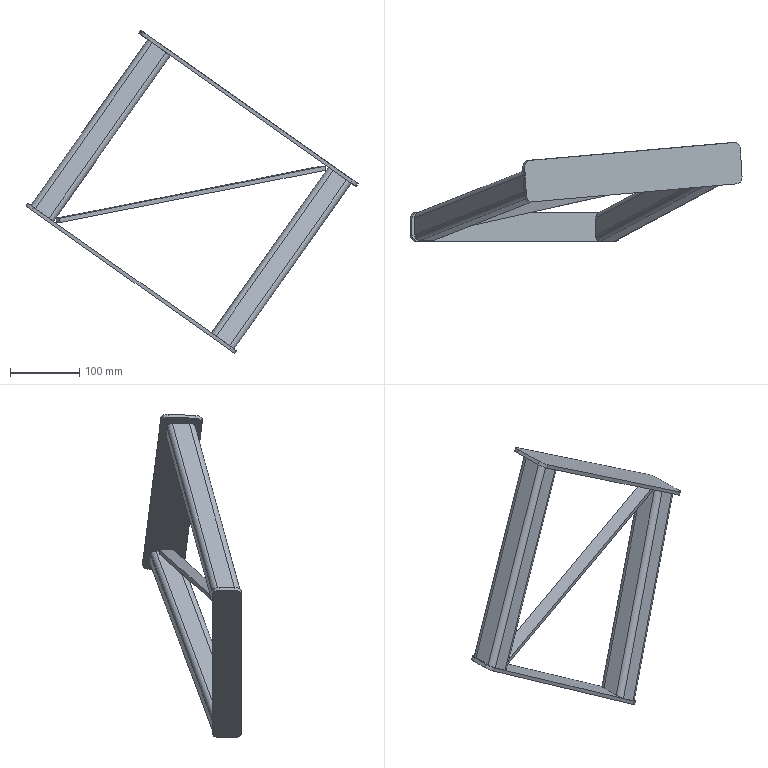Part | STEP file | upper-lower conveyor link bracket left | 5 solids | 62 faces | box 480.245 x 142.878 x 467.818 mm | volume 564874 mm3 | plane 38 | cylinder 24 | commonest cylinder face diameters 8 x8 16 x8 20 x8